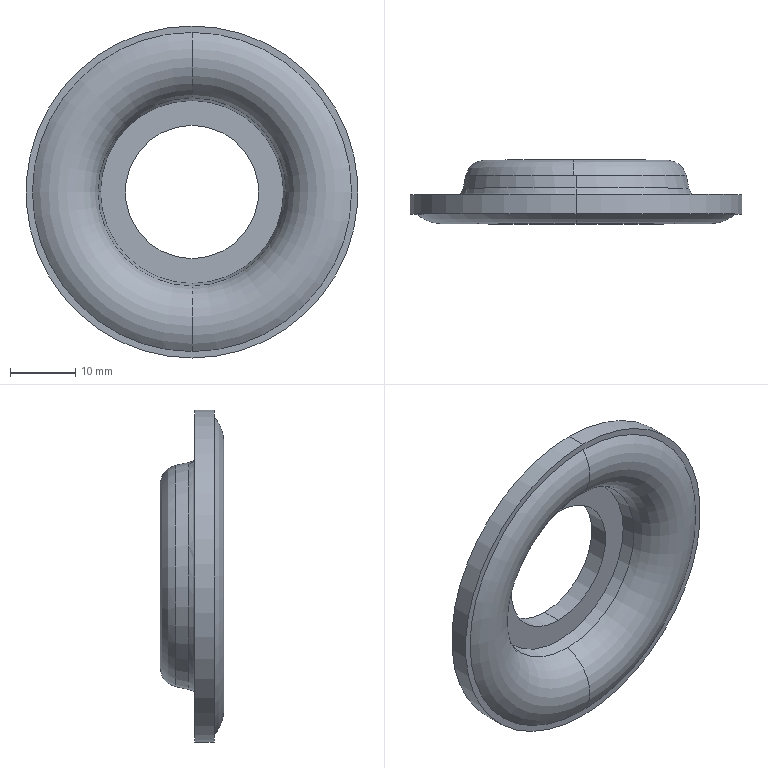Part | NX | features solid 2 | 1 solid | 18 faces | box 51.05 x 9.8 x 51.05 mm | volume 6527 mm3 | torus 6 | cone 4 | plane 4 | cylinder 4 | commonest cylinder face diameters 20.5 x2 51.05 x2
STEP:
#1=CARTESIAN_POINT('',(189.638,-21.474,-119.997));
#2=VERTEX_POINT('',#1);
#3=CARTESIAN_POINT('',(190.,-21.474,-154.007));
#4=VERTEX_POINT('',#3);
#5=CARTESIAN_POINT('',(190.,-21.474,-137.));
#6=DIRECTION('',(0.,-1.,0.));
#7=DIRECTION('',(-0.02126,0.,0.9998));
#8=AXIS2_PLACEMENT_3D('',#5,#6,#7);
#9=CIRCLE('',#8,17.007);
#10=EDGE_CURVE('',#2,#4,#9,.T.);
#11=ORIENTED_EDGE('',*,*,#10,.T.);
#12=CARTESIAN_POINT('',(190.,-23.408,-154.419));
#13=VERTEX_POINT('',#12);
#14=CARTESIAN_POINT('',(190.,-23.408,-154.419));
#15=DIRECTION('',(0.,0.978,0.2087));
#16=VECTOR('',#15,1000.);
#17=LINE('',#14,#16);
#18=EDGE_CURVE('',#4,#13,#17,.F.);
#19=ORIENTED_EDGE('',*,*,#18,.T.);
#20=CARTESIAN_POINT('',(190.,-23.408,-119.581));
#21=VERTEX_POINT('',#20);
#22=CARTESIAN_POINT('',(190.,-23.408,-137.));
#23=DIRECTION('',(0.,1.,0.));
#24=DIRECTION('',(0.,0.,-1.));
#25=AXIS2_PLACEMENT_3D('',#22,#23,#24);
#26=CIRCLE('',#25,17.419);
#27=EDGE_CURVE('',#13,#21,#26,.T.);
#28=ORIENTED_EDGE('',*,*,#27,.T.);
#29=CARTESIAN_POINT('',(190.,-21.474,-119.993));
#30=VERTEX_POINT('',#29);
#31=CARTESIAN_POINT('',(190.,-23.408,-119.581));
#32=DIRECTION('',(0.,0.978,-0.2087));
#33=VECTOR('',#32,1000.);
#34=LINE('',#31,#33);
#35=EDGE_CURVE('',#21,#30,#34,.T.);
#36=ORIENTED_EDGE('',*,*,#35,.T.);
#37=CARTESIAN_POINT('',(190.,-21.474,-137.));
#38=DIRECTION('',(0.,-1.,0.));
#39=DIRECTION('',(0.,0.,1.));
#40=AXIS2_PLACEMENT_3D('',#37,#38,#39);
#41=CIRCLE('',#40,17.007);
#42=EDGE_CURVE('',#30,#2,#41,.T.);
#43=ORIENTED_EDGE('',*,*,#42,.T.);
#44=EDGE_LOOP('',(#11,#19,#28,#36,#43));
#45=FACE_BOUND('',#44,.T.);
#46=CARTESIAN_POINT('',(190.,-22.441,-137.));
#47=DIRECTION('',(0.,-1.,0.));
#48=DIRECTION('',(0.,0.,-1.));
#49=AXIS2_PLACEMENT_3D('',#46,#47,#48);
#50=CONICAL_SURFACE('',#49,17.213,0.2103);
#51=ADVANCED_FACE('',(#45),#50,.T.);
#52=ORIENTED_EDGE('',*,*,#42,.F.);
#53=CARTESIAN_POINT('',(190.362,-21.474,-154.003));
#54=VERTEX_POINT('',#53);
#55=CARTESIAN_POINT('',(190.,-21.474,-137.));
#56=DIRECTION('',(0.,-1.,0.));
#57=DIRECTION('',(0.02126,0.,-0.9998));
#58=AXIS2_PLACEMENT_3D('',#55,#56,#57);
#59=CIRCLE('',#58,17.007);
#60=EDGE_CURVE('',#54,#30,#59,.T.);
#61=ORIENTED_EDGE('',*,*,#60,.F.);
#62=CARTESIAN_POINT('',(190.299,-19.1,-151.07));
#63=VERTEX_POINT('',#62);
#64=CARTESIAN_POINT('',(190.299,-22.1,-151.07));
#65=DIRECTION('',(-0.9998,0.,-0.02126));
#66=DIRECTION('',(-0.000000006,1.,0.00000026));
#67=AXIS2_PLACEMENT_3D('',#64,#65,#66);
#68=CIRCLE('',#67,3.);
#69=EDGE_CURVE('',#63,#54,#68,.T.);
#70=ORIENTED_EDGE('',*,*,#69,.F.);
#71=CARTESIAN_POINT('',(190.008,-19.1,-122.928));
#72=VERTEX_POINT('',#71);
#73=CARTESIAN_POINT('',(190.,-19.1,-137.));
#74=DIRECTION('',(0.,-1.,0.));
#75=DIRECTION('',(0.02126,0.,-0.9998));
#76=AXIS2_PLACEMENT_3D('',#73,#74,#75);
#77=CIRCLE('',#76,14.073);
#78=EDGE_CURVE('',#72,#63,#77,.F.);
#79=ORIENTED_EDGE('',*,*,#78,.F.);
#80=CARTESIAN_POINT('',(189.701,-19.1,-122.93));
#81=VERTEX_POINT('',#80);
#82=CARTESIAN_POINT('',(190.,-19.1,-137.));
#83=DIRECTION('',(0.,1.,0.));
#84=DIRECTION('',(-0.02126,0.,0.9998));
#85=AXIS2_PLACEMENT_3D('',#82,#83,#84);
#86=CIRCLE('',#85,14.072);
#87=EDGE_CURVE('',#81,#72,#86,.T.);
#88=ORIENTED_EDGE('',*,*,#87,.F.);
#89=CARTESIAN_POINT('',(189.701,-22.1,-122.93));
#90=DIRECTION('',(0.9998,0.,0.02126));
#91=DIRECTION('',(0.000000005,1.,-0.000000244));
#92=AXIS2_PLACEMENT_3D('',#89,#90,#91);
#93=CIRCLE('',#92,3.);
#94=EDGE_CURVE('',#2,#81,#93,.F.);
#95=ORIENTED_EDGE('',*,*,#94,.F.);
#96=EDGE_LOOP('',(#52,#61,#70,#79,#88,#95));
#97=FACE_BOUND('',#96,.T.);
#98=CARTESIAN_POINT('',(190.,-22.1,-137.));
#99=DIRECTION('',(0.,1.,0.));
#100=DIRECTION('',(-0.02126,0.,0.9998));
#101=AXIS2_PLACEMENT_3D('',#98,#99,#100);
#102=TOROIDAL_SURFACE('',#101,14.073,3.);
#103=ADVANCED_FACE('',(#97),#102,.T.);
#104=ORIENTED_EDGE('',*,*,#94,.T.);
#105=CARTESIAN_POINT('',(189.992,-19.1,-151.072));
#106=VERTEX_POINT('',#105);
#107=CARTESIAN_POINT('',(190.,-19.1,-137.));
#108=DIRECTION('',(0.,-1.,0.));
#109=DIRECTION('',(-0.02126,0.,0.9998));
#110=AXIS2_PLACEMENT_3D('',#107,#108,#109);
#111=CIRCLE('',#110,14.073);
#112=EDGE_CURVE('',#106,#81,#111,.F.);
#113=ORIENTED_EDGE('',*,*,#112,.F.);
#114=CARTESIAN_POINT('',(190.,-19.1,-137.));
#115=DIRECTION('',(0.,1.,0.));
#116=DIRECTION('',(0.02126,0.,-0.9998));
#117=AXIS2_PLACEMENT_3D('',#114,#115,#116);
#118=CIRCLE('',#117,14.072);
#119=EDGE_CURVE('',#63,#106,#118,.T.);
#120=ORIENTED_EDGE('',*,*,#119,.F.);
#121=ORIENTED_EDGE('',*,*,#69,.T.);
#122=CARTESIAN_POINT('',(190.,-21.474,-137.));
#123=DIRECTION('',(0.,-1.,0.));
#124=DIRECTION('',(0.,0.,-1.));
#125=AXIS2_PLACEMENT_3D('',#122,#123,#124);
#126=CIRCLE('',#125,17.007);
#127=EDGE_CURVE('',#4,#54,#126,.T.);
#128=ORIENTED_EDGE('',*,*,#127,.F.);
#129=ORIENTED_EDGE('',*,*,#10,.F.);
#130=EDGE_LOOP('',(#104,#113,#120,#121,#128,#129));
#131=FACE_BOUND('',#130,.T.);
#132=CARTESIAN_POINT('',(190.,-22.1,-137.));
#133=DIRECTION('',(0.,1.,0.));
#134=DIRECTION('',(0.02126,0.,-0.9998));
#135=AXIS2_PLACEMENT_3D('',#132,#133,#134);
#136=TOROIDAL_SURFACE('',#135,14.073,3.);
#137=ADVANCED_FACE('',(#131),#136,.T.);
#138=ORIENTED_EDGE('',*,*,#127,.T.);
#139=ORIENTED_EDGE('',*,*,#60,.T.);
#140=ORIENTED_EDGE('',*,*,#35,.F.);
#141=CARTESIAN_POINT('',(190.,-23.408,-137.));
#142=DIRECTION('',(0.,1.,0.));
#143=DIRECTION('',(0.,0.,1.));
#144=AXIS2_PLACEMENT_3D('',#141,#142,#143);
#145=CIRCLE('',#144,17.419);
#146=EDGE_CURVE('',#21,#13,#145,.T.);
#147=ORIENTED_EDGE('',*,*,#146,.T.);
#148=ORIENTED_EDGE('',*,*,#18,.F.);
#149=EDGE_LOOP('',(#138,#139,#140,#147,#148));
#150=FACE_BOUND('',#149,.T.);
#151=CARTESIAN_POINT('',(190.,-22.441,-137.));
#152=DIRECTION('',(0.,-1.,0.));
#153=DIRECTION('',(0.,0.,-1.));
#154=AXIS2_PLACEMENT_3D('',#151,#152,#153);
#155=CONICAL_SURFACE('',#154,17.213,0.2103);
#156=ADVANCED_FACE('',(#150),#155,.T.);
#157=CARTESIAN_POINT('',(190.,-24.4,-113.817));
#158=VERTEX_POINT('',#157);
#159=CARTESIAN_POINT('',(190.,-22.75,-116.5));
#160=DIRECTION('',(1.,0.,0.));
#161=DIRECTION('',(0.,-0.5238,0.8518));
#162=AXIS2_PLACEMENT_3D('',#159,#160,#161);
#163=CIRCLE('',#162,3.15);
#164=EDGE_CURVE('',#21,#158,#163,.F.);
#165=ORIENTED_EDGE('',*,*,#164,.T.);
#166=CARTESIAN_POINT('',(190.,-24.4,-160.183));
#167=VERTEX_POINT('',#166);
#168=CARTESIAN_POINT('',(190.,-24.4,-137.));
#169=DIRECTION('',(0.,1.,0.));
#170=DIRECTION('',(0.,0.,1.));
#171=AXIS2_PLACEMENT_3D('',#168,#169,#170);
#172=CIRCLE('',#171,23.183);
#173=EDGE_CURVE('',#158,#167,#172,.T.);
#174=ORIENTED_EDGE('',*,*,#173,.T.);
#175=CARTESIAN_POINT('',(190.,-22.75,-157.5));
#176=DIRECTION('',(-1.,0.,0.));
#177=DIRECTION('',(0.,-0.5238,-0.8518));
#178=AXIS2_PLACEMENT_3D('',#175,#176,#177);
#179=CIRCLE('',#178,3.15);
#180=EDGE_CURVE('',#167,#13,#179,.T.);
#181=ORIENTED_EDGE('',*,*,#180,.T.);
#182=ORIENTED_EDGE('',*,*,#146,.F.);
#183=EDGE_LOOP('',(#165,#174,#181,#182));
#184=FACE_BOUND('',#183,.T.);
#185=CARTESIAN_POINT('',(190.,-22.75,-137.));
#186=DIRECTION('',(0.,-1.,0.));
#187=DIRECTION('',(0.,0.,1.));
#188=AXIS2_PLACEMENT_3D('',#185,#186,#187);
#189=TOROIDAL_SURFACE('',#188,20.5,3.15);
#190=ADVANCED_FACE('',(#184),#189,.F.);
#191=ORIENTED_EDGE('',*,*,#27,.F.);
#192=ORIENTED_EDGE('',*,*,#180,.F.);
#193=CARTESIAN_POINT('',(190.,-24.4,-137.));
#194=DIRECTION('',(0.,1.,0.));
#195=DIRECTION('',(0.,0.,-1.));
#196=AXIS2_PLACEMENT_3D('',#193,#194,#195);
#197=CIRCLE('',#196,23.183);
#198=EDGE_CURVE('',#167,#158,#197,.T.);
#199=ORIENTED_EDGE('',*,*,#198,.T.);
#200=ORIENTED_EDGE('',*,*,#164,.F.);
#201=EDGE_LOOP('',(#191,#192,#199,#200));
#202=FACE_BOUND('',#201,.T.);
#203=CARTESIAN_POINT('',(190.,-22.75,-137.));
#204=DIRECTION('',(0.,-1.,0.));
#205=DIRECTION('',(0.,0.,-1.));
#206=AXIS2_PLACEMENT_3D('',#203,#204,#205);
#207=TOROIDAL_SURFACE('',#206,20.5,3.15);
#208=ADVANCED_FACE('',(#202),#207,.F.);
#209=CARTESIAN_POINT('',(190.,-24.4,-162.525));
#210=VERTEX_POINT('',#209);
#211=CARTESIAN_POINT('',(190.,-24.4,-111.475));
#212=VERTEX_POINT('',#211);
#213=CARTESIAN_POINT('',(190.,-24.4,-137.));
#214=DIRECTION('',(0.,-1.,0.));
#215=DIRECTION('',(0.,0.,-1.));
#216=AXIS2_PLACEMENT_3D('',#213,#214,#215);
#217=CIRCLE('',#216,25.525);
#218=EDGE_CURVE('',#210,#212,#217,.T.);
#219=ORIENTED_EDGE('',*,*,#218,.F.);
#220=CARTESIAN_POINT('',(190.,-24.4,-137.));
#221=DIRECTION('',(0.,-1.,0.));
#222=DIRECTION('',(0.,0.,1.));
#223=AXIS2_PLACEMENT_3D('',#220,#221,#222);
#224=CIRCLE('',#223,25.525);
#225=EDGE_CURVE('',#212,#210,#224,.T.);
#226=ORIENTED_EDGE('',*,*,#225,.F.);
#227=EDGE_LOOP('',(#219,#226));
#228=FACE_BOUND('',#227,.T.);
#229=ORIENTED_EDGE('',*,*,#173,.F.);
#230=ORIENTED_EDGE('',*,*,#198,.F.);
#231=EDGE_LOOP('',(#229,#230));
#232=FACE_BOUND('',#231,.T.);
#233=CARTESIAN_POINT('',(190.,-24.4,-137.));
#234=DIRECTION('',(0.,-1.,0.));
#235=DIRECTION('',(0.,0.,-1.));
#236=AXIS2_PLACEMENT_3D('',#233,#234,#235);
#237=PLANE('',#236);
#238=ADVANCED_FACE('',(#228,#232),#237,.F.);
#239=CARTESIAN_POINT('',(190.,-27.4,-162.525));
#240=VERTEX_POINT('',#239);
#241=CARTESIAN_POINT('',(190.,-27.4,-162.525));
#242=DIRECTION('',(0.,1.,0.));
#243=VECTOR('',#242,1000.);
#244=LINE('',#241,#243);
#245=EDGE_CURVE('',#210,#240,#244,.F.);
#246=ORIENTED_EDGE('',*,*,#245,.T.);
#247=CARTESIAN_POINT('',(190.,-27.4,-111.475));
#248=VERTEX_POINT('',#247);
#249=CARTESIAN_POINT('',(190.,-27.4,-137.));
#250=DIRECTION('',(0.,1.,0.));
#251=DIRECTION('',(0.,0.,-1.));
#252=AXIS2_PLACEMENT_3D('',#249,#250,#251);
#253=CIRCLE('',#252,25.525);
#254=EDGE_CURVE('',#240,#248,#253,.T.);
#255=ORIENTED_EDGE('',*,*,#254,.T.);
#256=CARTESIAN_POINT('',(190.,-27.4,-111.475));
#257=DIRECTION('',(0.,1.,0.));
#258=VECTOR('',#257,1000.);
#259=LINE('',#256,#258);
#260=EDGE_CURVE('',#248,#212,#259,.T.);
#261=ORIENTED_EDGE('',*,*,#260,.T.);
#262=ORIENTED_EDGE('',*,*,#225,.T.);
#263=EDGE_LOOP('',(#246,#255,#261,#262));
#264=FACE_BOUND('',#263,.T.);
#265=CARTESIAN_POINT('',(190.,-18.61,-137.));
#266=DIRECTION('',(0.,-1.,0.));
#267=DIRECTION('',(0.,0.,-1.));
#268=AXIS2_PLACEMENT_3D('',#265,#266,#267);
#269=CYLINDRICAL_SURFACE('',#268,25.525);
#270=ADVANCED_FACE('',(#264),#269,.T.);
#271=ORIENTED_EDGE('',*,*,#218,.T.);
#272=ORIENTED_EDGE('',*,*,#260,.F.);
#273=CARTESIAN_POINT('',(190.,-27.4,-137.));
#274=DIRECTION('',(0.,1.,0.));
#275=DIRECTION('',(0.,0.,1.));
#276=AXIS2_PLACEMENT_3D('',#273,#274,#275);
#277=CIRCLE('',#276,25.525);
#278=EDGE_CURVE('',#248,#240,#277,.T.);
#279=ORIENTED_EDGE('',*,*,#278,.T.);
#280=ORIENTED_EDGE('',*,*,#245,.F.);
#281=EDGE_LOOP('',(#271,#272,#279,#280));
#282=FACE_BOUND('',#281,.T.);
#283=CARTESIAN_POINT('',(190.,-18.61,-137.));
#284=DIRECTION('',(0.,-1.,0.));
#285=DIRECTION('',(0.,0.,-1.));
#286=AXIS2_PLACEMENT_3D('',#283,#284,#285);
#287=CYLINDRICAL_SURFACE('',#286,25.525);
#288=ADVANCED_FACE('',(#282),#287,.T.);
#289=ORIENTED_EDGE('',*,*,#278,.F.);
#290=ORIENTED_EDGE('',*,*,#254,.F.);
#291=EDGE_LOOP('',(#289,#290));
#292=FACE_BOUND('',#291,.T.);
#293=CARTESIAN_POINT('',(190.,-27.4,-112.475));
#294=VERTEX_POINT('',#293);
#295=CARTESIAN_POINT('',(190.,-27.4,-161.525));
#296=VERTEX_POINT('',#295);
#297=CARTESIAN_POINT('',(190.,-27.4,-137.));
#298=DIRECTION('',(0.,-1.,0.));
#299=DIRECTION('',(0.,0.,1.));
#300=AXIS2_PLACEMENT_3D('',#297,#298,#299);
#301=CIRCLE('',#300,24.525);
#302=EDGE_CURVE('',#294,#296,#301,.T.);
#303=ORIENTED_EDGE('',*,*,#302,.F.);
#304=CARTESIAN_POINT('',(190.,-27.4,-137.));
#305=DIRECTION('',(0.,-1.,0.));
#306=DIRECTION('',(0.,0.,-1.));
#307=AXIS2_PLACEMENT_3D('',#304,#305,#306);
#308=CIRCLE('',#307,24.525);
#309=EDGE_CURVE('',#296,#294,#308,.T.);
#310=ORIENTED_EDGE('',*,*,#309,.F.);
#311=EDGE_LOOP('',(#303,#310));
#312=FACE_BOUND('',#311,.T.);
#313=CARTESIAN_POINT('',(190.,-27.4,-137.));
#314=DIRECTION('',(0.,-1.,0.));
#315=DIRECTION('',(0.,0.,-1.));
#316=AXIS2_PLACEMENT_3D('',#313,#314,#315);
#317=PLANE('',#316);
#318=ADVANCED_FACE('',(#292,#312),#317,.T.);
#319=CARTESIAN_POINT('',(204.485,-24.034,-137.));
#320=VERTEX_POINT('',#319);
#321=CARTESIAN_POINT('',(190.,-24.034,-122.515));
#322=VERTEX_POINT('',#321);
#323=CARTESIAN_POINT('',(190.,-24.034,-137.));
#324=DIRECTION('',(0.,-1.,0.));
#325=DIRECTION('',(1.,0.,0.));
#326=AXIS2_PLACEMENT_3D('',#323,#324,#325);
#327=CIRCLE('',#326,14.485);
#328=EDGE_CURVE('',#320,#322,#327,.T.);
#329=ORIENTED_EDGE('',*,*,#328,.F.);
#330=CARTESIAN_POINT('',(190.,-24.034,-151.485));
#331=VERTEX_POINT('',#330);
#332=CARTESIAN_POINT('',(190.,-24.034,-137.));
#333=DIRECTION('',(0.,-1.,0.));
#334=DIRECTION('',(0.,0.,-1.));
#335=AXIS2_PLACEMENT_3D('',#332,#333,#334);
#336=CIRCLE('',#335,14.485);
#337=EDGE_CURVE('',#331,#320,#336,.T.);
#338=ORIENTED_EDGE('',*,*,#337,.F.);
#339=CARTESIAN_POINT('',(190.,-22.75,-157.5));
#340=DIRECTION('',(-1.,0.,0.));
#341=DIRECTION('',(0.,-0.7561,-0.6545));
#342=AXIS2_PLACEMENT_3D('',#339,#340,#341);
#343=CIRCLE('',#342,6.15);
#344=EDGE_CURVE('',#296,#331,#343,.T.);
#345=ORIENTED_EDGE('',*,*,#344,.F.);
#346=ORIENTED_EDGE('',*,*,#309,.T.);
#347=CARTESIAN_POINT('',(190.,-22.75,-116.5));
#348=DIRECTION('',(1.,0.,0.));
#349=DIRECTION('',(0.,-0.7561,0.6545));
#350=AXIS2_PLACEMENT_3D('',#347,#348,#349);
#351=CIRCLE('',#350,6.15);
#352=EDGE_CURVE('',#322,#294,#351,.F.);
#353=ORIENTED_EDGE('',*,*,#352,.F.);
#354=EDGE_LOOP('',(#329,#338,#345,#346,#353));
#355=FACE_BOUND('',#354,.T.);
#356=CARTESIAN_POINT('',(190.,-22.75,-137.));
#357=DIRECTION('',(0.,-1.,0.));
#358=DIRECTION('',(0.,0.,1.));
#359=AXIS2_PLACEMENT_3D('',#356,#357,#358);
#360=TOROIDAL_SURFACE('',#359,20.5,6.15);
#361=ADVANCED_FACE('',(#355),#360,.T.);
#362=ORIENTED_EDGE('',*,*,#352,.T.);
#363=ORIENTED_EDGE('',*,*,#302,.T.);
#364=ORIENTED_EDGE('',*,*,#344,.T.);
#365=CARTESIAN_POINT('',(175.515,-24.034,-137.));
#366=VERTEX_POINT('',#365);
#367=CARTESIAN_POINT('',(190.,-24.034,-137.));
#368=DIRECTION('',(0.,-1.,0.));
#369=DIRECTION('',(-1.,0.,0.));
#370=AXIS2_PLACEMENT_3D('',#367,#368,#369);
#371=CIRCLE('',#370,14.485);
#372=EDGE_CURVE('',#366,#331,#371,.T.);
#373=ORIENTED_EDGE('',*,*,#372,.F.);
#374=CARTESIAN_POINT('',(190.,-24.034,-137.));
#375=DIRECTION('',(0.,-1.,0.));
#376=DIRECTION('',(0.,0.,1.));
#377=AXIS2_PLACEMENT_3D('',#374,#375,#376);
#378=CIRCLE('',#377,14.485);
#379=EDGE_CURVE('',#322,#366,#378,.T.);
#380=ORIENTED_EDGE('',*,*,#379,.F.);
#381=EDGE_LOOP('',(#362,#363,#364,#373,#380));
#382=FACE_BOUND('',#381,.T.);
#383=CARTESIAN_POINT('',(190.,-22.75,-137.));
#384=DIRECTION('',(0.,-1.,0.));
#385=DIRECTION('',(0.,0.,-1.));
#386=AXIS2_PLACEMENT_3D('',#383,#384,#385);
#387=TOROIDAL_SURFACE('',#386,20.5,6.15);
#388=ADVANCED_FACE('',(#382),#387,.T.);
#389=CARTESIAN_POINT('',(175.927,-22.1,-137.));
#390=VERTEX_POINT('',#389);
#391=CARTESIAN_POINT('',(204.073,-22.1,-137.));
#392=VERTEX_POINT('',#391);
#393=CARTESIAN_POINT('',(190.,-22.1,-137.));
#394=DIRECTION('',(0.,1.,0.));
#395=DIRECTION('',(-1.,0.,0.));
#396=AXIS2_PLACEMENT_3D('',#393,#394,#395);
#397=CIRCLE('',#396,14.073);
#398=EDGE_CURVE('',#390,#392,#397,.T.);
#399=ORIENTED_EDGE('',*,*,#398,.T.);
#400=CARTESIAN_POINT('',(204.485,-24.034,-137.));
#401=DIRECTION('',(-0.2087,0.978,0.));
#402=VECTOR('',#401,1000.);
#403=LINE('',#400,#402);
#404=EDGE_CURVE('',#320,#392,#403,.T.);
#405=ORIENTED_EDGE('',*,*,#404,.F.);
#406=ORIENTED_EDGE('',*,*,#328,.T.);
#407=ORIENTED_EDGE('',*,*,#379,.T.);
#408=CARTESIAN_POINT('',(175.515,-24.034,-137.));
#409=DIRECTION('',(0.2087,0.978,0.));
#410=VECTOR('',#409,1000.);
#411=LINE('',#408,#410);
#412=EDGE_CURVE('',#390,#366,#411,.F.);
#413=ORIENTED_EDGE('',*,*,#412,.F.);
#414=EDGE_LOOP('',(#399,#405,#406,#407,#413));
#415=FACE_BOUND('',#414,.T.);
#416=CARTESIAN_POINT('',(190.,-23.067,-137.));
#417=DIRECTION('',(0.,-1.,0.));
#418=DIRECTION('',(-1.,0.,0.));
#419=AXIS2_PLACEMENT_3D('',#416,#417,#418);
#420=CONICAL_SURFACE('',#419,14.279,0.2103);
#421=ADVANCED_FACE('',(#415),#420,.F.);
#422=ORIENTED_EDGE('',*,*,#412,.T.);
#423=ORIENTED_EDGE('',*,*,#372,.T.);
#424=ORIENTED_EDGE('',*,*,#337,.T.);
#425=ORIENTED_EDGE('',*,*,#404,.T.);
#426=CARTESIAN_POINT('',(190.,-22.1,-137.));
#427=DIRECTION('',(0.,1.,0.));
#428=DIRECTION('',(1.,0.,0.));
#429=AXIS2_PLACEMENT_3D('',#426,#427,#428);
#430=CIRCLE('',#429,14.073);
#431=EDGE_CURVE('',#392,#390,#430,.T.);
#432=ORIENTED_EDGE('',*,*,#431,.T.);
#433=EDGE_LOOP('',(#422,#423,#424,#425,#432));
#434=FACE_BOUND('',#433,.T.);
#435=CARTESIAN_POINT('',(190.,-23.067,-137.));
#436=DIRECTION('',(0.,-1.,0.));
#437=DIRECTION('',(-1.,0.,0.));
#438=AXIS2_PLACEMENT_3D('',#435,#436,#437);
#439=CONICAL_SURFACE('',#438,14.279,0.2103);
#440=ADVANCED_FACE('',(#434),#439,.F.);
#441=ORIENTED_EDGE('',*,*,#431,.F.);
#442=ORIENTED_EDGE('',*,*,#398,.F.);
#443=EDGE_LOOP('',(#441,#442));
#444=FACE_BOUND('',#443,.T.);
#445=CARTESIAN_POINT('',(190.,-22.1,-147.25));
#446=VERTEX_POINT('',#445);
#447=CARTESIAN_POINT('',(190.,-22.1,-126.75));
#448=VERTEX_POINT('',#447);
#449=CARTESIAN_POINT('',(190.,-22.1,-137.));
#450=DIRECTION('',(0.,-1.,0.));
#451=DIRECTION('',(0.,0.,-1.));
#452=AXIS2_PLACEMENT_3D('',#449,#450,#451);
#453=CIRCLE('',#452,10.25);
#454=EDGE_CURVE('',#446,#448,#453,.T.);
#455=ORIENTED_EDGE('',*,*,#454,.F.);
#456=CARTESIAN_POINT('',(190.,-22.1,-137.));
#457=DIRECTION('',(0.,-1.,0.));
#458=DIRECTION('',(0.,0.,1.));
#459=AXIS2_PLACEMENT_3D('',#456,#457,#458);
#460=CIRCLE('',#459,10.25);
#461=EDGE_CURVE('',#448,#446,#460,.T.);
#462=ORIENTED_EDGE('',*,*,#461,.F.);
#463=EDGE_LOOP('',(#455,#462));
#464=FACE_BOUND('',#463,.T.);
#465=CARTESIAN_POINT('',(190.,-22.1,-137.));
#466=DIRECTION('',(0.,-1.,0.));
#467=DIRECTION('',(0.,0.,-1.));
#468=AXIS2_PLACEMENT_3D('',#465,#466,#467);
#469=PLANE('',#468);
#470=ADVANCED_FACE('',(#444,#464),#469,.T.);
#471=ORIENTED_EDGE('',*,*,#461,.T.);
#472=CARTESIAN_POINT('',(190.,-19.1,-147.25));
#473=VERTEX_POINT('',#472);
#474=CARTESIAN_POINT('',(190.,-19.1,-147.25));
#475=DIRECTION('',(0.,-1.,0.));
#476=VECTOR('',#475,1000.);
#477=LINE('',#474,#476);
#478=EDGE_CURVE('',#446,#473,#477,.F.);
#479=ORIENTED_EDGE('',*,*,#478,.T.);
#480=CARTESIAN_POINT('',(190.,-19.1,-126.75));
#481=VERTEX_POINT('',#480);
#482=CARTESIAN_POINT('',(190.,-19.1,-137.));
#483=DIRECTION('',(0.,1.,0.));
#484=DIRECTION('',(0.,0.,-1.));
#485=AXIS2_PLACEMENT_3D('',#482,#483,#484);
#486=CIRCLE('',#485,10.25);
#487=EDGE_CURVE('',#473,#481,#486,.T.);
#488=ORIENTED_EDGE('',*,*,#487,.T.);
#489=CARTESIAN_POINT('',(190.,-19.1,-126.75));
#490=DIRECTION('',(0.,-1.,0.));
#491=VECTOR('',#490,1000.);
#492=LINE('',#489,#491);
#493=EDGE_CURVE('',#481,#448,#492,.T.);
#494=ORIENTED_EDGE('',*,*,#493,.T.);
#495=EDGE_LOOP('',(#471,#479,#488,#494));
#496=FACE_BOUND('',#495,.T.);
#497=CARTESIAN_POINT('',(190.,-19.1,-137.));
#498=DIRECTION('',(0.,1.,0.));
#499=DIRECTION('',(0.,0.,1.));
#500=AXIS2_PLACEMENT_3D('',#497,#498,#499);
#501=CYLINDRICAL_SURFACE('',#500,10.25);
#502=ADVANCED_FACE('',(#496),#501,.F.);
#503=ORIENTED_EDGE('',*,*,#493,.F.);
#504=CARTESIAN_POINT('',(190.,-19.1,-137.));
#505=DIRECTION('',(0.,1.,0.));
#506=DIRECTION('',(0.,0.,1.));
#507=AXIS2_PLACEMENT_3D('',#504,#505,#506);
#508=CIRCLE('',#507,10.25);
#509=EDGE_CURVE('',#481,#473,#508,.T.);
#510=ORIENTED_EDGE('',*,*,#509,.T.);
#511=ORIENTED_EDGE('',*,*,#478,.F.);
#512=ORIENTED_EDGE('',*,*,#454,.T.);
#513=EDGE_LOOP('',(#503,#510,#511,#512));
#514=FACE_BOUND('',#513,.T.);
#515=CARTESIAN_POINT('',(190.,-19.1,-137.));
#516=DIRECTION('',(0.,1.,0.));
#517=DIRECTION('',(0.,0.,1.));
#518=AXIS2_PLACEMENT_3D('',#515,#516,#517);
#519=CYLINDRICAL_SURFACE('',#518,10.25);
#520=ADVANCED_FACE('',(#514),#519,.F.);
#521=ORIENTED_EDGE('',*,*,#78,.T.);
#522=ORIENTED_EDGE('',*,*,#119,.T.);
#523=ORIENTED_EDGE('',*,*,#112,.T.);
#524=ORIENTED_EDGE('',*,*,#87,.T.);
#525=EDGE_LOOP('',(#521,#522,#523,#524));
#526=FACE_BOUND('',#525,.T.);
#527=ORIENTED_EDGE('',*,*,#487,.F.);
#528=ORIENTED_EDGE('',*,*,#509,.F.);
#529=EDGE_LOOP('',(#527,#528));
#530=FACE_BOUND('',#529,.T.);
#531=CARTESIAN_POINT('',(190.,-19.1,-137.));
#532=DIRECTION('',(0.,-1.,0.));
#533=DIRECTION('',(0.,0.,-1.));
#534=AXIS2_PLACEMENT_3D('',#531,#532,#533);
#535=PLANE('',#534);
#536=ADVANCED_FACE('',(#526,#530),#535,.F.);
#537=CLOSED_SHELL('',(#51,#103,#137,#156,#190,#208,#238,#270,#288,#318,#361,#388,#421,#440,#470,#502,#520,#536));
#538=MANIFOLD_SOLID_BREP('',#537);
#539=(LENGTH_UNIT()NAMED_UNIT(*)SI_UNIT(.MILLI.,.METRE.));
#540=UNCERTAINTY_MEASURE_WITH_UNIT(LENGTH_MEASURE(0.00001),#539,'','');
#541=(NAMED_UNIT(*)PLANE_ANGLE_UNIT()SI_UNIT($,.RADIAN.));
#542=(NAMED_UNIT(*)SI_UNIT($,.STERADIAN.)SOLID_ANGLE_UNIT());
#543=(GEOMETRIC_REPRESENTATION_CONTEXT(3)GLOBAL_UNCERTAINTY_ASSIGNED_CONTEXT((#540))GLOBAL_UNIT_ASSIGNED_CONTEXT((#539,#541,#542))REPRESENTATION_CONTEXT('',''));
#544=ADVANCED_BREP_SHAPE_REPRESENTATION('',(#538),#543);